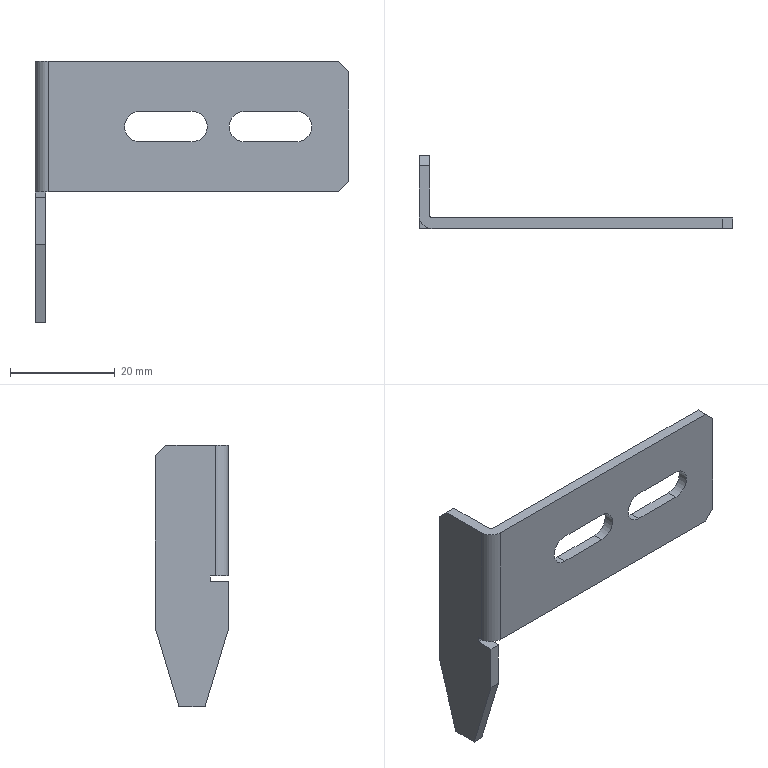Part | SolidWorks | features BaseBody 1 | 1 solid | 27 faces | box 60 x 14 x 50 mm | volume 3776 mm3 | plane 21 | cylinder 6 | commonest cylinder face diameters 5.8 x4 1 x1 5 x1
STEP:
#1=CARTESIAN_POINT('',(267.247,579.,-397.245));
#2=VERTEX_POINT('',#1);
#3=CARTESIAN_POINT('',(257.247,579.,-397.245));
#4=VERTEX_POINT('',#3);
#5=CARTESIAN_POINT('',(217.247,579.,-397.245));
#6=DIRECTION('',(-1.,0.,0.));
#7=VECTOR('',#6,1000.);
#8=LINE('',#5,#7);
#9=EDGE_CURVE('',#2,#4,#8,.T.);
#10=ORIENTED_EDGE('',*,*,#9,.F.);
#11=CARTESIAN_POINT('',(267.247,579.,-391.445));
#12=VERTEX_POINT('',#11);
#13=CARTESIAN_POINT('',(267.247,579.,-394.345));
#14=DIRECTION('',(0.,1.,0.));
#15=DIRECTION('',(0.,0.,1.));
#16=AXIS2_PLACEMENT_3D('',#13,#14,#15);
#17=CIRCLE('',#16,2.9);
#18=EDGE_CURVE('',#12,#2,#17,.T.);
#19=ORIENTED_EDGE('',*,*,#18,.F.);
#20=CARTESIAN_POINT('',(257.247,579.,-391.445));
#21=VERTEX_POINT('',#20);
#22=CARTESIAN_POINT('',(217.247,579.,-391.445));
#23=DIRECTION('',(1.,0.,0.));
#24=VECTOR('',#23,1000.);
#25=LINE('',#22,#24);
#26=EDGE_CURVE('',#21,#12,#25,.T.);
#27=ORIENTED_EDGE('',*,*,#26,.F.);
#28=CARTESIAN_POINT('',(257.247,579.,-394.345));
#29=DIRECTION('',(0.,1.,0.));
#30=DIRECTION('',(0.,0.,1.));
#31=AXIS2_PLACEMENT_3D('',#28,#29,#30);
#32=CIRCLE('',#31,2.9);
#33=EDGE_CURVE('',#4,#21,#32,.T.);
#34=ORIENTED_EDGE('',*,*,#33,.F.);
#35=EDGE_LOOP('',(#10,#19,#27,#34));
#36=FACE_BOUND('',#35,.T.);
#37=CARTESIAN_POINT('',(247.247,579.,-397.245));
#38=VERTEX_POINT('',#37);
#39=CARTESIAN_POINT('',(237.247,579.,-397.245));
#40=VERTEX_POINT('',#39);
#41=CARTESIAN_POINT('',(217.247,579.,-397.245));
#42=DIRECTION('',(-1.,0.,0.));
#43=VECTOR('',#42,1000.);
#44=LINE('',#41,#43);
#45=EDGE_CURVE('',#38,#40,#44,.T.);
#46=ORIENTED_EDGE('',*,*,#45,.F.);
#47=CARTESIAN_POINT('',(247.247,579.,-391.445));
#48=VERTEX_POINT('',#47);
#49=CARTESIAN_POINT('',(247.247,579.,-394.345));
#50=DIRECTION('',(0.,1.,0.));
#51=DIRECTION('',(0.,0.,1.));
#52=AXIS2_PLACEMENT_3D('',#49,#50,#51);
#53=CIRCLE('',#52,2.9);
#54=EDGE_CURVE('',#48,#38,#53,.T.);
#55=ORIENTED_EDGE('',*,*,#54,.F.);
#56=CARTESIAN_POINT('',(237.247,579.,-391.445));
#57=VERTEX_POINT('',#56);
#58=CARTESIAN_POINT('',(217.247,579.,-391.445));
#59=DIRECTION('',(1.,0.,0.));
#60=VECTOR('',#59,1000.);
#61=LINE('',#58,#60);
#62=EDGE_CURVE('',#57,#48,#61,.T.);
#63=ORIENTED_EDGE('',*,*,#62,.F.);
#64=CARTESIAN_POINT('',(237.247,579.,-394.345));
#65=DIRECTION('',(0.,1.,0.));
#66=DIRECTION('',(0.,0.,1.));
#67=AXIS2_PLACEMENT_3D('',#64,#65,#66);
#68=CIRCLE('',#67,2.9);
#69=EDGE_CURVE('',#40,#57,#68,.T.);
#70=ORIENTED_EDGE('',*,*,#69,.F.);
#71=EDGE_LOOP('',(#46,#55,#63,#70));
#72=FACE_BOUND('',#71,.T.);
#73=CARTESIAN_POINT('',(219.747,579.,-406.845));
#74=VERTEX_POINT('',#73);
#75=CARTESIAN_POINT('',(275.247,579.,-406.845));
#76=VERTEX_POINT('',#75);
#77=CARTESIAN_POINT('',(217.247,579.,-406.845));
#78=DIRECTION('',(1.,0.,0.));
#79=VECTOR('',#78,1000.);
#80=LINE('',#77,#79);
#81=EDGE_CURVE('',#74,#76,#80,.T.);
#82=ORIENTED_EDGE('',*,*,#81,.F.);
#83=CARTESIAN_POINT('',(219.747,579.,-381.845));
#84=VERTEX_POINT('',#83);
#85=CARTESIAN_POINT('',(219.747,579.,-431.845));
#86=DIRECTION('',(0.,0.,-1.));
#87=VECTOR('',#86,1000.);
#88=LINE('',#85,#87);
#89=EDGE_CURVE('',#84,#74,#88,.T.);
#90=ORIENTED_EDGE('',*,*,#89,.F.);
#91=CARTESIAN_POINT('',(275.247,579.,-381.845));
#92=VERTEX_POINT('',#91);
#93=CARTESIAN_POINT('',(217.247,579.,-381.845));
#94=DIRECTION('',(-1.,0.,0.));
#95=VECTOR('',#94,1000.);
#96=LINE('',#93,#95);
#97=EDGE_CURVE('',#92,#84,#96,.T.);
#98=ORIENTED_EDGE('',*,*,#97,.F.);
#99=CARTESIAN_POINT('',(277.247,579.,-383.845));
#100=VERTEX_POINT('',#99);
#101=CARTESIAN_POINT('',(277.247,579.,-383.845));
#102=DIRECTION('',(-0.7071,0.,0.7071));
#103=VECTOR('',#102,1000.);
#104=LINE('',#101,#103);
#105=EDGE_CURVE('',#100,#92,#104,.T.);
#106=ORIENTED_EDGE('',*,*,#105,.F.);
#107=CARTESIAN_POINT('',(277.247,579.,-404.845));
#108=VERTEX_POINT('',#107);
#109=CARTESIAN_POINT('',(277.247,579.,-431.845));
#110=DIRECTION('',(0.,0.,1.));
#111=VECTOR('',#110,1000.);
#112=LINE('',#109,#111);
#113=EDGE_CURVE('',#108,#100,#112,.T.);
#114=ORIENTED_EDGE('',*,*,#113,.F.);
#115=CARTESIAN_POINT('',(275.247,579.,-406.845));
#116=DIRECTION('',(0.7071,0.,0.7071));
#117=VECTOR('',#116,1000.);
#118=LINE('',#115,#117);
#119=EDGE_CURVE('',#76,#108,#118,.T.);
#120=ORIENTED_EDGE('',*,*,#119,.F.);
#121=EDGE_LOOP('',(#82,#90,#98,#106,#114,#120));
#122=FACE_OUTER_BOUND('',#121,.T.);
#123=CARTESIAN_POINT('',(217.247,579.,-431.845));
#124=DIRECTION('',(0.,-1.,0.));
#125=DIRECTION('',(0.,0.,-1.));
#126=AXIS2_PLACEMENT_3D('',#123,#124,#125);
#127=PLANE('',#126);
#128=ADVANCED_FACE('',(#36,#72,#122),#127,.F.);
#129=CARTESIAN_POINT('',(257.247,577.,-397.245));
#130=VERTEX_POINT('',#129);
#131=CARTESIAN_POINT('',(257.247,579.,-397.245));
#132=DIRECTION('',(0.,-1.,0.));
#133=VECTOR('',#132,1000.);
#134=LINE('',#131,#133);
#135=EDGE_CURVE('',#4,#130,#134,.T.);
#136=ORIENTED_EDGE('',*,*,#135,.F.);
#137=ORIENTED_EDGE('',*,*,#33,.T.);
#138=CARTESIAN_POINT('',(257.247,577.,-391.445));
#139=VERTEX_POINT('',#138);
#140=CARTESIAN_POINT('',(257.247,579.,-391.445));
#141=DIRECTION('',(0.,1.,0.));
#142=VECTOR('',#141,1000.);
#143=LINE('',#140,#142);
#144=EDGE_CURVE('',#139,#21,#143,.T.);
#145=ORIENTED_EDGE('',*,*,#144,.F.);
#146=CARTESIAN_POINT('',(257.247,577.,-394.345));
#147=DIRECTION('',(0.,1.,0.));
#148=DIRECTION('',(0.,0.,1.));
#149=AXIS2_PLACEMENT_3D('',#146,#147,#148);
#150=CIRCLE('',#149,2.9);
#151=EDGE_CURVE('',#130,#139,#150,.T.);
#152=ORIENTED_EDGE('',*,*,#151,.F.);
#153=EDGE_LOOP('',(#136,#137,#145,#152));
#154=FACE_OUTER_BOUND('',#153,.T.);
#155=CARTESIAN_POINT('',(257.247,579.,-394.345));
#156=DIRECTION('',(0.,1.,0.));
#157=DIRECTION('',(0.,0.,1.));
#158=AXIS2_PLACEMENT_3D('',#155,#156,#157);
#159=CYLINDRICAL_SURFACE('',#158,2.9);
#160=ADVANCED_FACE('',(#154),#159,.F.);
#161=ORIENTED_EDGE('',*,*,#9,.T.);
#162=ORIENTED_EDGE('',*,*,#135,.T.);
#163=CARTESIAN_POINT('',(267.247,577.,-397.245));
#164=VERTEX_POINT('',#163);
#165=CARTESIAN_POINT('',(267.247,577.,-397.245));
#166=DIRECTION('',(-1.,0.,0.));
#167=VECTOR('',#166,1000.);
#168=LINE('',#165,#167);
#169=EDGE_CURVE('',#164,#130,#168,.T.);
#170=ORIENTED_EDGE('',*,*,#169,.F.);
#171=CARTESIAN_POINT('',(267.247,579.,-397.245));
#172=DIRECTION('',(0.,-1.,0.));
#173=VECTOR('',#172,1000.);
#174=LINE('',#171,#173);
#175=EDGE_CURVE('',#2,#164,#174,.T.);
#176=ORIENTED_EDGE('',*,*,#175,.F.);
#177=EDGE_LOOP('',(#161,#162,#170,#176));
#178=FACE_OUTER_BOUND('',#177,.T.);
#179=CARTESIAN_POINT('',(267.247,579.,-397.245));
#180=DIRECTION('',(0.,0.,-1.));
#181=DIRECTION('',(-1.,0.,0.));
#182=AXIS2_PLACEMENT_3D('',#179,#180,#181);
#183=PLANE('',#182);
#184=ADVANCED_FACE('',(#178),#183,.F.);
#185=ORIENTED_EDGE('',*,*,#18,.T.);
#186=ORIENTED_EDGE('',*,*,#175,.T.);
#187=CARTESIAN_POINT('',(267.247,577.,-391.445));
#188=VERTEX_POINT('',#187);
#189=CARTESIAN_POINT('',(267.247,577.,-394.345));
#190=DIRECTION('',(0.,1.,0.));
#191=DIRECTION('',(0.,0.,1.));
#192=AXIS2_PLACEMENT_3D('',#189,#190,#191);
#193=CIRCLE('',#192,2.9);
#194=EDGE_CURVE('',#188,#164,#193,.T.);
#195=ORIENTED_EDGE('',*,*,#194,.F.);
#196=CARTESIAN_POINT('',(267.247,579.,-391.445));
#197=DIRECTION('',(0.,-1.,0.));
#198=VECTOR('',#197,1000.);
#199=LINE('',#196,#198);
#200=EDGE_CURVE('',#12,#188,#199,.T.);
#201=ORIENTED_EDGE('',*,*,#200,.F.);
#202=EDGE_LOOP('',(#185,#186,#195,#201));
#203=FACE_OUTER_BOUND('',#202,.T.);
#204=CARTESIAN_POINT('',(267.247,579.,-394.345));
#205=DIRECTION('',(0.,1.,0.));
#206=DIRECTION('',(0.,0.,1.));
#207=AXIS2_PLACEMENT_3D('',#204,#205,#206);
#208=CYLINDRICAL_SURFACE('',#207,2.9);
#209=ADVANCED_FACE('',(#203),#208,.F.);
#210=ORIENTED_EDGE('',*,*,#26,.T.);
#211=ORIENTED_EDGE('',*,*,#200,.T.);
#212=CARTESIAN_POINT('',(267.247,577.,-391.445));
#213=DIRECTION('',(1.,0.,0.));
#214=VECTOR('',#213,1000.);
#215=LINE('',#212,#214);
#216=EDGE_CURVE('',#139,#188,#215,.T.);
#217=ORIENTED_EDGE('',*,*,#216,.F.);
#218=ORIENTED_EDGE('',*,*,#144,.T.);
#219=EDGE_LOOP('',(#210,#211,#217,#218));
#220=FACE_OUTER_BOUND('',#219,.T.);
#221=CARTESIAN_POINT('',(267.247,579.,-391.445));
#222=DIRECTION('',(0.,0.,1.));
#223=DIRECTION('',(1.,0.,0.));
#224=AXIS2_PLACEMENT_3D('',#221,#222,#223);
#225=PLANE('',#224);
#226=ADVANCED_FACE('',(#220),#225,.F.);
#227=ORIENTED_EDGE('',*,*,#45,.T.);
#228=CARTESIAN_POINT('',(237.247,577.,-397.245));
#229=VERTEX_POINT('',#228);
#230=CARTESIAN_POINT('',(237.247,579.,-397.245));
#231=DIRECTION('',(0.,1.,0.));
#232=VECTOR('',#231,1000.);
#233=LINE('',#230,#232);
#234=EDGE_CURVE('',#229,#40,#233,.T.);
#235=ORIENTED_EDGE('',*,*,#234,.F.);
#236=CARTESIAN_POINT('',(247.247,577.,-397.245));
#237=VERTEX_POINT('',#236);
#238=CARTESIAN_POINT('',(247.247,577.,-397.245));
#239=DIRECTION('',(-1.,0.,0.));
#240=VECTOR('',#239,1000.);
#241=LINE('',#238,#240);
#242=EDGE_CURVE('',#237,#229,#241,.T.);
#243=ORIENTED_EDGE('',*,*,#242,.F.);
#244=CARTESIAN_POINT('',(247.247,579.,-397.245));
#245=DIRECTION('',(0.,-1.,0.));
#246=VECTOR('',#245,1000.);
#247=LINE('',#244,#246);
#248=EDGE_CURVE('',#38,#237,#247,.T.);
#249=ORIENTED_EDGE('',*,*,#248,.F.);
#250=EDGE_LOOP('',(#227,#235,#243,#249));
#251=FACE_OUTER_BOUND('',#250,.T.);
#252=CARTESIAN_POINT('',(247.247,579.,-397.245));
#253=DIRECTION('',(0.,0.,-1.));
#254=DIRECTION('',(-1.,0.,0.));
#255=AXIS2_PLACEMENT_3D('',#252,#253,#254);
#256=PLANE('',#255);
#257=ADVANCED_FACE('',(#251),#256,.F.);
#258=ORIENTED_EDGE('',*,*,#54,.T.);
#259=ORIENTED_EDGE('',*,*,#248,.T.);
#260=CARTESIAN_POINT('',(247.247,577.,-391.445));
#261=VERTEX_POINT('',#260);
#262=CARTESIAN_POINT('',(247.247,577.,-394.345));
#263=DIRECTION('',(0.,1.,0.));
#264=DIRECTION('',(0.,0.,1.));
#265=AXIS2_PLACEMENT_3D('',#262,#263,#264);
#266=CIRCLE('',#265,2.9);
#267=EDGE_CURVE('',#261,#237,#266,.T.);
#268=ORIENTED_EDGE('',*,*,#267,.F.);
#269=CARTESIAN_POINT('',(247.247,579.,-391.445));
#270=DIRECTION('',(0.,-1.,0.));
#271=VECTOR('',#270,1000.);
#272=LINE('',#269,#271);
#273=EDGE_CURVE('',#48,#261,#272,.T.);
#274=ORIENTED_EDGE('',*,*,#273,.F.);
#275=EDGE_LOOP('',(#258,#259,#268,#274));
#276=FACE_OUTER_BOUND('',#275,.T.);
#277=CARTESIAN_POINT('',(247.247,579.,-394.345));
#278=DIRECTION('',(0.,1.,0.));
#279=DIRECTION('',(0.,0.,1.));
#280=AXIS2_PLACEMENT_3D('',#277,#278,#279);
#281=CYLINDRICAL_SURFACE('',#280,2.9);
#282=ADVANCED_FACE('',(#276),#281,.F.);
#283=ORIENTED_EDGE('',*,*,#62,.T.);
#284=ORIENTED_EDGE('',*,*,#273,.T.);
#285=CARTESIAN_POINT('',(237.247,577.,-391.445));
#286=VERTEX_POINT('',#285);
#287=CARTESIAN_POINT('',(247.247,577.,-391.445));
#288=DIRECTION('',(1.,0.,0.));
#289=VECTOR('',#288,1000.);
#290=LINE('',#287,#289);
#291=EDGE_CURVE('',#286,#261,#290,.T.);
#292=ORIENTED_EDGE('',*,*,#291,.F.);
#293=CARTESIAN_POINT('',(237.247,579.,-391.445));
#294=DIRECTION('',(0.,-1.,0.));
#295=VECTOR('',#294,1000.);
#296=LINE('',#293,#295);
#297=EDGE_CURVE('',#57,#286,#296,.T.);
#298=ORIENTED_EDGE('',*,*,#297,.F.);
#299=EDGE_LOOP('',(#283,#284,#292,#298));
#300=FACE_OUTER_BOUND('',#299,.T.);
#301=CARTESIAN_POINT('',(247.247,579.,-391.445));
#302=DIRECTION('',(0.,0.,1.));
#303=DIRECTION('',(1.,0.,0.));
#304=AXIS2_PLACEMENT_3D('',#301,#302,#303);
#305=PLANE('',#304);
#306=ADVANCED_FACE('',(#300),#305,.F.);
#307=ORIENTED_EDGE('',*,*,#234,.T.);
#308=ORIENTED_EDGE('',*,*,#69,.T.);
#309=ORIENTED_EDGE('',*,*,#297,.T.);
#310=CARTESIAN_POINT('',(237.247,577.,-394.345));
#311=DIRECTION('',(0.,1.,0.));
#312=DIRECTION('',(0.,0.,1.));
#313=AXIS2_PLACEMENT_3D('',#310,#311,#312);
#314=CIRCLE('',#313,2.9);
#315=EDGE_CURVE('',#229,#286,#314,.T.);
#316=ORIENTED_EDGE('',*,*,#315,.F.);
#317=EDGE_LOOP('',(#307,#308,#309,#316));
#318=FACE_OUTER_BOUND('',#317,.T.);
#319=CARTESIAN_POINT('',(237.247,579.,-394.345));
#320=DIRECTION('',(0.,1.,0.));
#321=DIRECTION('',(0.,0.,1.));
#322=AXIS2_PLACEMENT_3D('',#319,#320,#321);
#323=CYLINDRICAL_SURFACE('',#322,2.9);
#324=ADVANCED_FACE('',(#318),#323,.F.);
#325=ORIENTED_EDGE('',*,*,#119,.T.);
#326=CARTESIAN_POINT('',(277.247,577.,-404.845));
#327=VERTEX_POINT('',#326);
#328=CARTESIAN_POINT('',(277.247,577.,-404.845));
#329=DIRECTION('',(0.,1.,0.));
#330=VECTOR('',#329,1000.);
#331=LINE('',#328,#330);
#332=EDGE_CURVE('',#327,#108,#331,.T.);
#333=ORIENTED_EDGE('',*,*,#332,.F.);
#334=CARTESIAN_POINT('',(275.247,577.,-406.845));
#335=VERTEX_POINT('',#334);
#336=CARTESIAN_POINT('',(277.247,577.,-404.845));
#337=DIRECTION('',(0.7071,0.,0.7071));
#338=VECTOR('',#337,1000.);
#339=LINE('',#336,#338);
#340=EDGE_CURVE('',#335,#327,#339,.T.);
#341=ORIENTED_EDGE('',*,*,#340,.F.);
#342=CARTESIAN_POINT('',(275.247,577.,-406.845));
#343=DIRECTION('',(0.,-1.,0.));
#344=VECTOR('',#343,1000.);
#345=LINE('',#342,#344);
#346=EDGE_CURVE('',#76,#335,#345,.T.);
#347=ORIENTED_EDGE('',*,*,#346,.F.);
#348=EDGE_LOOP('',(#325,#333,#341,#347));
#349=FACE_OUTER_BOUND('',#348,.T.);
#350=CARTESIAN_POINT('',(277.247,577.,-404.845));
#351=DIRECTION('',(-0.7071,0.,0.7071));
#352=DIRECTION('',(0.7071,0.,0.7071));
#353=AXIS2_PLACEMENT_3D('',#350,#351,#352);
#354=PLANE('',#353);
#355=ADVANCED_FACE('',(#349),#354,.F.);
#356=CARTESIAN_POINT('',(219.747,577.,-406.845));
#357=VERTEX_POINT('',#356);
#358=CARTESIAN_POINT('',(219.247,577.,-406.845));
#359=DIRECTION('',(-1.,0.,0.));
#360=VECTOR('',#359,1000.);
#361=LINE('',#358,#360);
#362=EDGE_CURVE('',#335,#357,#361,.T.);
#363=ORIENTED_EDGE('',*,*,#362,.T.);
#364=CARTESIAN_POINT('',(217.247,579.5,-406.845));
#365=VERTEX_POINT('',#364);
#366=CARTESIAN_POINT('',(219.747,579.5,-406.845));
#367=DIRECTION('',(0.,0.,1.));
#368=DIRECTION('',(-1.,0.,0.));
#369=AXIS2_PLACEMENT_3D('',#366,#367,#368);
#370=CIRCLE('',#369,2.5);
#371=EDGE_CURVE('',#365,#357,#370,.T.);
#372=ORIENTED_EDGE('',*,*,#371,.F.);
#373=CARTESIAN_POINT('',(217.247,580.5,-406.845));
#374=VERTEX_POINT('',#373);
#375=CARTESIAN_POINT('',(217.247,580.5,-406.845));
#376=DIRECTION('',(0.,1.,0.));
#377=VECTOR('',#376,1000.);
#378=LINE('',#375,#377);
#379=EDGE_CURVE('',#365,#374,#378,.T.);
#380=ORIENTED_EDGE('',*,*,#379,.T.);
#381=CARTESIAN_POINT('',(219.247,580.5,-406.845));
#382=VERTEX_POINT('',#381);
#383=CARTESIAN_POINT('',(219.247,580.5,-406.845));
#384=DIRECTION('',(1.,0.,0.));
#385=VECTOR('',#384,1000.);
#386=LINE('',#383,#385);
#387=EDGE_CURVE('',#374,#382,#386,.T.);
#388=ORIENTED_EDGE('',*,*,#387,.T.);
#389=CARTESIAN_POINT('',(219.247,579.5,-406.845));
#390=VERTEX_POINT('',#389);
#391=CARTESIAN_POINT('',(219.247,584.,-406.845));
#392=DIRECTION('',(0.,-1.,0.));
#393=VECTOR('',#392,1000.);
#394=LINE('',#391,#393);
#395=EDGE_CURVE('',#382,#390,#394,.T.);
#396=ORIENTED_EDGE('',*,*,#395,.T.);
#397=CARTESIAN_POINT('',(219.747,579.5,-406.845));
#398=DIRECTION('',(0.,0.,1.));
#399=DIRECTION('',(-1.,0.,0.));
#400=AXIS2_PLACEMENT_3D('',#397,#398,#399);
#401=CIRCLE('',#400,0.5);
#402=EDGE_CURVE('',#390,#74,#401,.T.);
#403=ORIENTED_EDGE('',*,*,#402,.T.);
#404=ORIENTED_EDGE('',*,*,#81,.T.);
#405=ORIENTED_EDGE('',*,*,#346,.T.);
#406=EDGE_LOOP('',(#363,#372,#380,#388,#396,#403,#404,#405));
#407=FACE_OUTER_BOUND('',#406,.T.);
#408=CARTESIAN_POINT('',(219.247,577.,-406.845));
#409=DIRECTION('',(0.,0.,-1.));
#410=DIRECTION('',(-1.,0.,0.));
#411=AXIS2_PLACEMENT_3D('',#408,#409,#410);
#412=PLANE('',#411);
#413=ADVANCED_FACE('',(#407),#412,.T.);
#414=ORIENTED_EDGE('',*,*,#89,.T.);
#415=ORIENTED_EDGE('',*,*,#402,.F.);
#416=CARTESIAN_POINT('',(219.247,579.5,-381.845));
#417=VERTEX_POINT('',#416);
#418=CARTESIAN_POINT('',(219.247,579.5,-406.845));
#419=DIRECTION('',(0.,0.,-1.));
#420=VECTOR('',#419,1000.);
#421=LINE('',#418,#420);
#422=EDGE_CURVE('',#417,#390,#421,.T.);
#423=ORIENTED_EDGE('',*,*,#422,.F.);
#424=CARTESIAN_POINT('',(219.747,579.5,-381.845));
#425=DIRECTION('',(0.,0.,-1.));
#426=DIRECTION('',(-1.,0.,0.));
#427=AXIS2_PLACEMENT_3D('',#424,#425,#426);
#428=CIRCLE('',#427,0.5);
#429=EDGE_CURVE('',#84,#417,#428,.T.);
#430=ORIENTED_EDGE('',*,*,#429,.F.);
#431=EDGE_LOOP('',(#414,#415,#423,#430));
#432=FACE_OUTER_BOUND('',#431,.T.);
#433=CARTESIAN_POINT('',(219.747,579.5,-406.845));
#434=DIRECTION('',(0.,0.,-1.));
#435=DIRECTION('',(-1.,0.,0.));
#436=AXIS2_PLACEMENT_3D('',#433,#434,#435);
#437=CYLINDRICAL_SURFACE('',#436,0.5);
#438=ADVANCED_FACE('',(#432),#437,.F.);
#439=ORIENTED_EDGE('',*,*,#97,.T.);
#440=ORIENTED_EDGE('',*,*,#429,.T.);
#441=CARTESIAN_POINT('',(219.247,589.,-381.845));
#442=VERTEX_POINT('',#441);
#443=CARTESIAN_POINT('',(219.247,584.,-381.845));
#444=DIRECTION('',(0.,1.,0.));
#445=VECTOR('',#444,1000.);
#446=LINE('',#443,#445);
#447=EDGE_CURVE('',#417,#442,#446,.T.);
#448=ORIENTED_EDGE('',*,*,#447,.T.);
#449=CARTESIAN_POINT('',(217.247,589.,-381.845));
#450=VERTEX_POINT('',#449);
#451=CARTESIAN_POINT('',(219.247,589.,-381.845));
#452=DIRECTION('',(-1.,0.,0.));
#453=VECTOR('',#452,1000.);
#454=LINE('',#451,#453);
#455=EDGE_CURVE('',#442,#450,#454,.T.);
#456=ORIENTED_EDGE('',*,*,#455,.T.);
#457=CARTESIAN_POINT('',(217.247,579.5,-381.845));
#458=VERTEX_POINT('',#457);
#459=CARTESIAN_POINT('',(217.247,577.,-381.845));
#460=DIRECTION('',(0.,-1.,0.));
#461=VECTOR('',#460,1000.);
#462=LINE('',#459,#461);
#463=EDGE_CURVE('',#450,#458,#462,.T.);
#464=ORIENTED_EDGE('',*,*,#463,.T.);
#465=CARTESIAN_POINT('',(219.747,577.,-381.845));
#466=VERTEX_POINT('',#465);
#467=CARTESIAN_POINT('',(219.747,579.5,-381.845));
#468=DIRECTION('',(0.,0.,1.));
#469=DIRECTION('',(-1.,0.,0.));
#470=AXIS2_PLACEMENT_3D('',#467,#468,#469);
#471=CIRCLE('',#470,2.5);
#472=EDGE_CURVE('',#458,#466,#471,.T.);
#473=ORIENTED_EDGE('',*,*,#472,.T.);
#474=CARTESIAN_POINT('',(275.247,577.,-381.845));
#475=VERTEX_POINT('',#474);
#476=CARTESIAN_POINT('',(277.247,577.,-381.845));
#477=DIRECTION('',(1.,0.,0.));
#478=VECTOR('',#477,1000.);
#479=LINE('',#476,#478);
#480=EDGE_CURVE('',#466,#475,#479,.T.);
#481=ORIENTED_EDGE('',*,*,#480,.T.);
#482=CARTESIAN_POINT('',(275.247,577.,-381.845));
#483=DIRECTION('',(0.,1.,0.));
#484=VECTOR('',#483,1000.);
#485=LINE('',#482,#484);
#486=EDGE_CURVE('',#475,#92,#485,.T.);
#487=ORIENTED_EDGE('',*,*,#486,.T.);
#488=EDGE_LOOP('',(#439,#440,#448,#456,#464,#473,#481,#487));
#489=FACE_OUTER_BOUND('',#488,.T.);
#490=CARTESIAN_POINT('',(277.247,577.,-381.845));
#491=DIRECTION('',(0.,0.,1.));
#492=DIRECTION('',(1.,0.,0.));
#493=AXIS2_PLACEMENT_3D('',#490,#491,#492);
#494=PLANE('',#493);
#495=ADVANCED_FACE('',(#489),#494,.T.);
#496=ORIENTED_EDGE('',*,*,#105,.T.);
#497=ORIENTED_EDGE('',*,*,#486,.F.);
#498=CARTESIAN_POINT('',(277.247,577.,-383.845));
#499=VERTEX_POINT('',#498);
#500=CARTESIAN_POINT('',(275.247,577.,-381.845));
#501=DIRECTION('',(-0.7071,0.,0.7071));
#502=VECTOR('',#501,1000.);
#503=LINE('',#500,#502);
#504=EDGE_CURVE('',#499,#475,#503,.T.);
#505=ORIENTED_EDGE('',*,*,#504,.F.);
#506=CARTESIAN_POINT('',(277.247,577.,-383.845));
#507=DIRECTION('',(0.,-1.,0.));
#508=VECTOR('',#507,1000.);
#509=LINE('',#506,#508);
#510=EDGE_CURVE('',#100,#499,#509,.T.);
#511=ORIENTED_EDGE('',*,*,#510,.F.);
#512=EDGE_LOOP('',(#496,#497,#505,#511));
#513=FACE_OUTER_BOUND('',#512,.T.);
#514=CARTESIAN_POINT('',(275.247,577.,-381.845));
#515=DIRECTION('',(-0.7071,0.,-0.7071));
#516=DIRECTION('',(-0.7071,0.,0.7071));
#517=AXIS2_PLACEMENT_3D('',#514,#515,#516);
#518=PLANE('',#517);
#519=ADVANCED_FACE('',(#513),#518,.F.);
#520=ORIENTED_EDGE('',*,*,#510,.T.);
#521=CARTESIAN_POINT('',(277.247,577.,-406.845));
#522=DIRECTION('',(0.,0.,-1.));
#523=VECTOR('',#522,1000.);
#524=LINE('',#521,#523);
#525=EDGE_CURVE('',#499,#327,#524,.T.);
#526=ORIENTED_EDGE('',*,*,#525,.T.);
#527=ORIENTED_EDGE('',*,*,#332,.T.);
#528=ORIENTED_EDGE('',*,*,#113,.T.);
#529=EDGE_LOOP('',(#520,#526,#527,#528));
#530=FACE_OUTER_BOUND('',#529,.T.);
#531=CARTESIAN_POINT('',(277.247,577.,-406.845));
#532=DIRECTION('',(1.,0.,0.));
#533=DIRECTION('',(0.,0.,-1.));
#534=AXIS2_PLACEMENT_3D('',#531,#532,#533);
#535=PLANE('',#534);
#536=ADVANCED_FACE('',(#530),#535,.T.);
#537=ORIENTED_EDGE('',*,*,#216,.T.);
#538=ORIENTED_EDGE('',*,*,#194,.T.);
#539=ORIENTED_EDGE('',*,*,#169,.T.);
#540=ORIENTED_EDGE('',*,*,#151,.T.);
#541=EDGE_LOOP('',(#537,#538,#539,#540));
#542=FACE_BOUND('',#541,.T.);
#543=ORIENTED_EDGE('',*,*,#315,.T.);
#544=ORIENTED_EDGE('',*,*,#291,.T.);
#545=ORIENTED_EDGE('',*,*,#267,.T.);
#546=ORIENTED_EDGE('',*,*,#242,.T.);
#547=EDGE_LOOP('',(#543,#544,#545,#546));
#548=FACE_BOUND('',#547,.T.);
#549=CARTESIAN_POINT('',(219.747,577.,-431.845));
#550=DIRECTION('',(0.,0.,-1.));
#551=VECTOR('',#550,1000.);
#552=LINE('',#549,#551);
#553=EDGE_CURVE('',#466,#357,#552,.T.);
#554=ORIENTED_EDGE('',*,*,#553,.T.);
#555=ORIENTED_EDGE('',*,*,#362,.F.);
#556=ORIENTED_EDGE('',*,*,#340,.T.);
#557=ORIENTED_EDGE('',*,*,#525,.F.);
#558=ORIENTED_EDGE('',*,*,#504,.T.);
#559=ORIENTED_EDGE('',*,*,#480,.F.);
#560=EDGE_LOOP('',(#554,#555,#556,#557,#558,#559));
#561=FACE_OUTER_BOUND('',#560,.T.);
#562=CARTESIAN_POINT('',(217.247,577.,-431.845));
#563=DIRECTION('',(0.,-1.,0.));
#564=DIRECTION('',(0.,0.,-1.));
#565=AXIS2_PLACEMENT_3D('',#562,#563,#564);
#566=PLANE('',#565);
#567=ADVANCED_FACE('',(#542,#548,#561),#566,.T.);
#568=ORIENTED_EDGE('',*,*,#447,.F.);
#569=ORIENTED_EDGE('',*,*,#422,.T.);
#570=ORIENTED_EDGE('',*,*,#395,.F.);
#571=CARTESIAN_POINT('',(219.247,580.5,-407.845));
#572=VERTEX_POINT('',#571);
#573=CARTESIAN_POINT('',(219.247,580.5,-431.845));
#574=DIRECTION('',(0.,0.,1.));
#575=VECTOR('',#574,1000.);
#576=LINE('',#573,#575);
#577=EDGE_CURVE('',#572,#382,#576,.T.);
#578=ORIENTED_EDGE('',*,*,#577,.F.);
#579=CARTESIAN_POINT('',(219.247,577.,-407.845));
#580=VERTEX_POINT('',#579);
#581=CARTESIAN_POINT('',(219.247,584.,-407.845));
#582=DIRECTION('',(0.,1.,0.));
#583=VECTOR('',#582,1000.);
#584=LINE('',#581,#583);
#585=EDGE_CURVE('',#580,#572,#584,.T.);
#586=ORIENTED_EDGE('',*,*,#585,.F.);
#587=CARTESIAN_POINT('',(219.247,577.,-416.845));
#588=VERTEX_POINT('',#587);
#589=CARTESIAN_POINT('',(219.247,577.,-431.845));
#590=DIRECTION('',(0.,0.,1.));
#591=VECTOR('',#590,1000.);
#592=LINE('',#589,#591);
#593=EDGE_CURVE('',#588,#580,#592,.T.);
#594=ORIENTED_EDGE('',*,*,#593,.F.);
#595=CARTESIAN_POINT('',(219.247,581.5,-431.845));
#596=VERTEX_POINT('',#595);
#597=CARTESIAN_POINT('',(219.247,581.5,-431.845));
#598=DIRECTION('',(0.,-0.2873,0.9578));
#599=VECTOR('',#598,1000.);
#600=LINE('',#597,#599);
#601=EDGE_CURVE('',#596,#588,#600,.T.);
#602=ORIENTED_EDGE('',*,*,#601,.F.);
#603=CARTESIAN_POINT('',(219.247,586.5,-431.845));
#604=VERTEX_POINT('',#603);
#605=CARTESIAN_POINT('',(219.247,584.,-431.845));
#606=DIRECTION('',(0.,-1.,0.));
#607=VECTOR('',#606,1000.);
#608=LINE('',#605,#607);
#609=EDGE_CURVE('',#604,#596,#608,.T.);
#610=ORIENTED_EDGE('',*,*,#609,.F.);
#611=CARTESIAN_POINT('',(219.247,591.,-416.845));
#612=VERTEX_POINT('',#611);
#613=CARTESIAN_POINT('',(219.247,591.,-416.845));
#614=DIRECTION('',(0.,-0.2873,-0.9578));
#615=VECTOR('',#614,1000.);
#616=LINE('',#613,#615);
#617=EDGE_CURVE('',#612,#604,#616,.T.);
#618=ORIENTED_EDGE('',*,*,#617,.F.);
#619=CARTESIAN_POINT('',(219.247,591.,-383.845));
#620=VERTEX_POINT('',#619);
#621=CARTESIAN_POINT('',(219.247,591.,-431.845));
#622=DIRECTION('',(0.,0.,-1.));
#623=VECTOR('',#622,1000.);
#624=LINE('',#621,#623);
#625=EDGE_CURVE('',#620,#612,#624,.T.);
#626=ORIENTED_EDGE('',*,*,#625,.F.);
#627=CARTESIAN_POINT('',(219.247,589.,-381.845));
#628=DIRECTION('',(0.,0.7071,-0.7071));
#629=VECTOR('',#628,1000.);
#630=LINE('',#627,#629);
#631=EDGE_CURVE('',#442,#620,#630,.T.);
#632=ORIENTED_EDGE('',*,*,#631,.F.);
#633=EDGE_LOOP('',(#568,#569,#570,#578,#586,#594,#602,#610,#618,#626,#632));
#634=FACE_OUTER_BOUND('',#633,.T.);
#635=CARTESIAN_POINT('',(219.247,584.,-431.845));
#636=DIRECTION('',(-1.,0.,0.));
#637=DIRECTION('',(0.,0.,1.));
#638=AXIS2_PLACEMENT_3D('',#635,#636,#637);
#639=PLANE('',#638);
#640=ADVANCED_FACE('',(#634),#639,.F.);
#641=ORIENTED_EDGE('',*,*,#472,.F.);
#642=CARTESIAN_POINT('',(217.247,579.5,-406.845));
#643=DIRECTION('',(0.,0.,-1.));
#644=VECTOR('',#643,1000.);
#645=LINE('',#642,#644);
#646=EDGE_CURVE('',#458,#365,#645,.T.);
#647=ORIENTED_EDGE('',*,*,#646,.T.);
#648=ORIENTED_EDGE('',*,*,#371,.T.);
#649=ORIENTED_EDGE('',*,*,#553,.F.);
#650=EDGE_LOOP('',(#641,#647,#648,#649));
#651=FACE_OUTER_BOUND('',#650,.T.);
#652=CARTESIAN_POINT('',(219.747,579.5,-406.845));
#653=DIRECTION('',(0.,0.,-1.));
#654=DIRECTION('',(-1.,0.,0.));
#655=AXIS2_PLACEMENT_3D('',#652,#653,#654);
#656=CYLINDRICAL_SURFACE('',#655,2.5);
#657=ADVANCED_FACE('',(#651),#656,.T.);
#658=CARTESIAN_POINT('',(217.247,591.,-383.845));
#659=VERTEX_POINT('',#658);
#660=CARTESIAN_POINT('',(217.247,589.,-381.845));
#661=DIRECTION('',(0.,0.7071,-0.7071));
#662=VECTOR('',#661,1000.);
#663=LINE('',#660,#662);
#664=EDGE_CURVE('',#450,#659,#663,.T.);
#665=ORIENTED_EDGE('',*,*,#664,.F.);
#666=ORIENTED_EDGE('',*,*,#455,.F.);
#667=ORIENTED_EDGE('',*,*,#631,.T.);
#668=CARTESIAN_POINT('',(219.247,591.,-383.845));
#669=DIRECTION('',(1.,0.,0.));
#670=VECTOR('',#669,1000.);
#671=LINE('',#668,#670);
#672=EDGE_CURVE('',#659,#620,#671,.T.);
#673=ORIENTED_EDGE('',*,*,#672,.F.);
#674=EDGE_LOOP('',(#665,#666,#667,#673));
#675=FACE_OUTER_BOUND('',#674,.T.);
#676=CARTESIAN_POINT('',(219.247,589.,-381.845));
#677=DIRECTION('',(0.,-0.7071,-0.7071));
#678=DIRECTION('',(0.,0.7071,-0.7071));
#679=AXIS2_PLACEMENT_3D('',#676,#677,#678);
#680=PLANE('',#679);
#681=ADVANCED_FACE('',(#675),#680,.F.);
#682=ORIENTED_EDGE('',*,*,#387,.F.);
#683=CARTESIAN_POINT('',(217.247,580.5,-407.845));
#684=VERTEX_POINT('',#683);
#685=CARTESIAN_POINT('',(217.247,580.5,-407.845));
#686=DIRECTION('',(0.,0.,-1.));
#687=VECTOR('',#686,1000.);
#688=LINE('',#685,#687);
#689=EDGE_CURVE('',#374,#684,#688,.T.);
#690=ORIENTED_EDGE('',*,*,#689,.T.);
#691=CARTESIAN_POINT('',(219.247,580.5,-407.845));
#692=DIRECTION('',(1.,0.,0.));
#693=VECTOR('',#692,1000.);
#694=LINE('',#691,#693);
#695=EDGE_CURVE('',#684,#572,#694,.T.);
#696=ORIENTED_EDGE('',*,*,#695,.T.);
#697=ORIENTED_EDGE('',*,*,#577,.T.);
#698=EDGE_LOOP('',(#682,#690,#696,#697));
#699=FACE_OUTER_BOUND('',#698,.T.);
#700=CARTESIAN_POINT('',(219.247,580.5,-407.845));
#701=DIRECTION('',(0.,-1.,0.));
#702=DIRECTION('',(0.,0.,-1.));
#703=AXIS2_PLACEMENT_3D('',#700,#701,#702);
#704=PLANE('',#703);
#705=ADVANCED_FACE('',(#699),#704,.T.);
#706=ORIENTED_EDGE('',*,*,#695,.F.);
#707=CARTESIAN_POINT('',(217.247,577.,-407.845));
#708=VERTEX_POINT('',#707);
#709=CARTESIAN_POINT('',(217.247,577.,-407.845));
#710=DIRECTION('',(0.,-1.,0.));
#711=VECTOR('',#710,1000.);
#712=LINE('',#709,#711);
#713=EDGE_CURVE('',#684,#708,#712,.T.);
#714=ORIENTED_EDGE('',*,*,#713,.T.);
#715=CARTESIAN_POINT('',(219.247,577.,-407.845));
#716=DIRECTION('',(1.,0.,0.));
#717=VECTOR('',#716,1000.);
#718=LINE('',#715,#717);
#719=EDGE_CURVE('',#708,#580,#718,.T.);
#720=ORIENTED_EDGE('',*,*,#719,.T.);
#721=ORIENTED_EDGE('',*,*,#585,.T.);
#722=EDGE_LOOP('',(#706,#714,#720,#721));
#723=FACE_OUTER_BOUND('',#722,.T.);
#724=CARTESIAN_POINT('',(219.247,577.,-407.845));
#725=DIRECTION('',(0.,0.,1.));
#726=DIRECTION('',(1.,0.,0.));
#727=AXIS2_PLACEMENT_3D('',#724,#725,#726);
#728=PLANE('',#727);
#729=ADVANCED_FACE('',(#723),#728,.T.);
#730=CARTESIAN_POINT('',(217.247,577.,-416.845));
#731=VERTEX_POINT('',#730);
#732=CARTESIAN_POINT('',(219.247,577.,-416.845));
#733=DIRECTION('',(1.,0.,0.));
#734=VECTOR('',#733,1000.);
#735=LINE('',#732,#734);
#736=EDGE_CURVE('',#731,#588,#735,.T.);
#737=ORIENTED_EDGE('',*,*,#736,.T.);
#738=ORIENTED_EDGE('',*,*,#593,.T.);
#739=ORIENTED_EDGE('',*,*,#719,.F.);
#740=CARTESIAN_POINT('',(217.247,577.,-416.845));
#741=DIRECTION('',(0.,0.,-1.));
#742=VECTOR('',#741,1000.);
#743=LINE('',#740,#742);
#744=EDGE_CURVE('',#708,#731,#743,.T.);
#745=ORIENTED_EDGE('',*,*,#744,.T.);
#746=EDGE_LOOP('',(#737,#738,#739,#745));
#747=FACE_OUTER_BOUND('',#746,.T.);
#748=CARTESIAN_POINT('',(219.247,577.,-416.845));
#749=DIRECTION('',(0.,-1.,0.));
#750=DIRECTION('',(0.,0.,-1.));
#751=AXIS2_PLACEMENT_3D('',#748,#749,#750);
#752=PLANE('',#751);
#753=ADVANCED_FACE('',(#747),#752,.T.);
#754=ORIENTED_EDGE('',*,*,#736,.F.);
#755=CARTESIAN_POINT('',(217.247,581.5,-431.845));
#756=VERTEX_POINT('',#755);
#757=CARTESIAN_POINT('',(217.247,581.5,-431.845));
#758=DIRECTION('',(0.,0.2873,-0.9578));
#759=VECTOR('',#758,1000.);
#760=LINE('',#757,#759);
#761=EDGE_CURVE('',#731,#756,#760,.T.);
#762=ORIENTED_EDGE('',*,*,#761,.T.);
#763=CARTESIAN_POINT('',(219.247,581.5,-431.845));
#764=DIRECTION('',(1.,0.,0.));
#765=VECTOR('',#764,1000.);
#766=LINE('',#763,#765);
#767=EDGE_CURVE('',#756,#596,#766,.T.);
#768=ORIENTED_EDGE('',*,*,#767,.T.);
#769=ORIENTED_EDGE('',*,*,#601,.T.);
#770=EDGE_LOOP('',(#754,#762,#768,#769));
#771=FACE_OUTER_BOUND('',#770,.T.);
#772=CARTESIAN_POINT('',(219.247,581.5,-431.845));
#773=DIRECTION('',(0.,-0.9578,-0.2873));
#774=DIRECTION('',(0.,0.2873,-0.9578));
#775=AXIS2_PLACEMENT_3D('',#772,#773,#774);
#776=PLANE('',#775);
#777=ADVANCED_FACE('',(#771),#776,.T.);
#778=ORIENTED_EDGE('',*,*,#767,.F.);
#779=CARTESIAN_POINT('',(217.247,586.5,-431.845));
#780=VERTEX_POINT('',#779);
#781=CARTESIAN_POINT('',(217.247,586.5,-431.845));
#782=DIRECTION('',(0.,1.,0.));
#783=VECTOR('',#782,1000.);
#784=LINE('',#781,#783);
#785=EDGE_CURVE('',#756,#780,#784,.T.);
#786=ORIENTED_EDGE('',*,*,#785,.T.);
#787=CARTESIAN_POINT('',(219.247,586.5,-431.845));
#788=DIRECTION('',(1.,0.,0.));
#789=VECTOR('',#788,1000.);
#790=LINE('',#787,#789);
#791=EDGE_CURVE('',#780,#604,#790,.T.);
#792=ORIENTED_EDGE('',*,*,#791,.T.);
#793=ORIENTED_EDGE('',*,*,#609,.T.);
#794=EDGE_LOOP('',(#778,#786,#792,#793));
#795=FACE_OUTER_BOUND('',#794,.T.);
#796=CARTESIAN_POINT('',(219.247,586.5,-431.845));
#797=DIRECTION('',(0.,0.,-1.));
#798=DIRECTION('',(-1.,0.,0.));
#799=AXIS2_PLACEMENT_3D('',#796,#797,#798);
#800=PLANE('',#799);
#801=ADVANCED_FACE('',(#795),#800,.T.);
#802=ORIENTED_EDGE('',*,*,#791,.F.);
#803=CARTESIAN_POINT('',(217.247,591.,-416.845));
#804=VERTEX_POINT('',#803);
#805=CARTESIAN_POINT('',(217.247,591.,-416.845));
#806=DIRECTION('',(0.,0.2873,0.9578));
#807=VECTOR('',#806,1000.);
#808=LINE('',#805,#807);
#809=EDGE_CURVE('',#780,#804,#808,.T.);
#810=ORIENTED_EDGE('',*,*,#809,.T.);
#811=CARTESIAN_POINT('',(219.247,591.,-416.845));
#812=DIRECTION('',(1.,0.,0.));
#813=VECTOR('',#812,1000.);
#814=LINE('',#811,#813);
#815=EDGE_CURVE('',#804,#612,#814,.T.);
#816=ORIENTED_EDGE('',*,*,#815,.T.);
#817=ORIENTED_EDGE('',*,*,#617,.T.);
#818=EDGE_LOOP('',(#802,#810,#816,#817));
#819=FACE_OUTER_BOUND('',#818,.T.);
#820=CARTESIAN_POINT('',(219.247,591.,-416.845));
#821=DIRECTION('',(0.,0.9578,-0.2873));
#822=DIRECTION('',(0.,0.2873,0.9578));
#823=AXIS2_PLACEMENT_3D('',#820,#821,#822);
#824=PLANE('',#823);
#825=ADVANCED_FACE('',(#819),#824,.T.);
#826=ORIENTED_EDGE('',*,*,#815,.F.);
#827=CARTESIAN_POINT('',(217.247,591.,-381.845));
#828=DIRECTION('',(0.,0.,1.));
#829=VECTOR('',#828,1000.);
#830=LINE('',#827,#829);
#831=EDGE_CURVE('',#804,#659,#830,.T.);
#832=ORIENTED_EDGE('',*,*,#831,.T.);
#833=ORIENTED_EDGE('',*,*,#672,.T.);
#834=ORIENTED_EDGE('',*,*,#625,.T.);
#835=EDGE_LOOP('',(#826,#832,#833,#834));
#836=FACE_OUTER_BOUND('',#835,.T.);
#837=CARTESIAN_POINT('',(219.247,591.,-381.845));
#838=DIRECTION('',(0.,1.,0.));
#839=DIRECTION('',(0.,0.,1.));
#840=AXIS2_PLACEMENT_3D('',#837,#838,#839);
#841=PLANE('',#840);
#842=ADVANCED_FACE('',(#836),#841,.T.);
#843=ORIENTED_EDGE('',*,*,#646,.F.);
#844=ORIENTED_EDGE('',*,*,#463,.F.);
#845=ORIENTED_EDGE('',*,*,#664,.T.);
#846=ORIENTED_EDGE('',*,*,#831,.F.);
#847=ORIENTED_EDGE('',*,*,#809,.F.);
#848=ORIENTED_EDGE('',*,*,#785,.F.);
#849=ORIENTED_EDGE('',*,*,#761,.F.);
#850=ORIENTED_EDGE('',*,*,#744,.F.);
#851=ORIENTED_EDGE('',*,*,#713,.F.);
#852=ORIENTED_EDGE('',*,*,#689,.F.);
#853=ORIENTED_EDGE('',*,*,#379,.F.);
#854=EDGE_LOOP('',(#843,#844,#845,#846,#847,#848,#849,#850,#851,#852,#853));
#855=FACE_OUTER_BOUND('',#854,.T.);
#856=CARTESIAN_POINT('',(217.247,584.,-431.845));
#857=DIRECTION('',(-1.,0.,0.));
#858=DIRECTION('',(0.,0.,1.));
#859=AXIS2_PLACEMENT_3D('',#856,#857,#858);
#860=PLANE('',#859);
#861=ADVANCED_FACE('',(#855),#860,.T.);
#862=CLOSED_SHELL('',(#128,#160,#184,#209,#226,#257,#282,#306,#324,#355,#413,#438,#495,#519,#536,#567,#640,#657,#681,#705,#729,#753,#777,#801,#825,#842,#861));
#863=MANIFOLD_SOLID_BREP('',#862);
#864=CARTESIAN_POINT('',(0.,0.,0.));
#865=DIRECTION('',(0.,0.,1.));
#866=DIRECTION('',(1.,0.,0.));
#867=AXIS2_PLACEMENT_3D('',#864,#865,#866);
#868=(LENGTH_UNIT()NAMED_UNIT(*)SI_UNIT(.MILLI.,.METRE.));
#869=UNCERTAINTY_MEASURE_WITH_UNIT(LENGTH_MEASURE(0.00001),#868,'','');
#870=(NAMED_UNIT(*)PLANE_ANGLE_UNIT()SI_UNIT($,.RADIAN.));
#871=(NAMED_UNIT(*)SI_UNIT($,.STERADIAN.)SOLID_ANGLE_UNIT());
#872=(GEOMETRIC_REPRESENTATION_CONTEXT(3)GLOBAL_UNCERTAINTY_ASSIGNED_CONTEXT((#869))GLOBAL_UNIT_ASSIGNED_CONTEXT((#868,#870,#871))REPRESENTATION_CONTEXT('',''));
#873=ADVANCED_BREP_SHAPE_REPRESENTATION('',(#863,#867),#872);